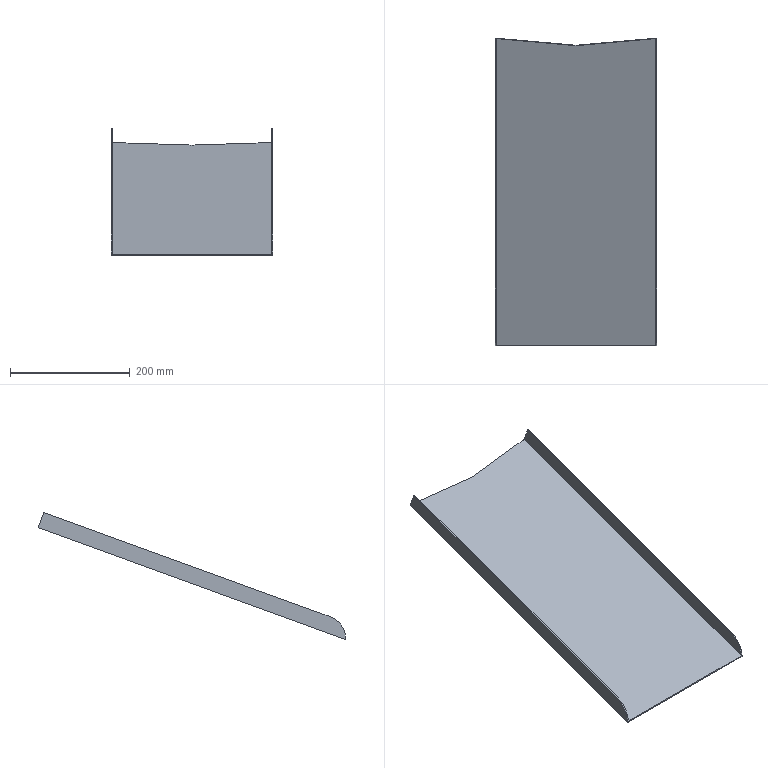Part | NX | features solid 2 | 1 solid | 17 faces | box 270 x 512.701 x 211.98 mm | volume 344500 mm3 | plane 15 | cylinder 2 | commonest cylinder face diameters 80 x2
STEP:
#1=CARTESIAN_POINT('',(133.,-620.,-424.26));
#2=VERTEX_POINT('',#1);
#3=CARTESIAN_POINT('',(-133.,-620.,-424.26));
#4=VERTEX_POINT('',#3);
#5=CARTESIAN_POINT('',(50.,-620.,-424.26));
#6=DIRECTION('',(1.,0.,0.));
#7=VECTOR('',#6,1000.);
#8=LINE('',#5,#7);
#9=EDGE_CURVE('',#2,#4,#8,.F.);
#10=ORIENTED_EDGE('',*,*,#9,.F.);
#11=CARTESIAN_POINT('',(133.,-108.158,-237.965));
#12=VERTEX_POINT('',#11);
#13=CARTESIAN_POINT('',(133.,-491.018,-377.315));
#14=DIRECTION('',(0.,-0.9397,-0.342));
#15=VECTOR('',#14,1000.);
#16=LINE('',#13,#15);
#17=EDGE_CURVE('',#12,#2,#16,.T.);
#18=ORIENTED_EDGE('',*,*,#17,.F.);
#19=CARTESIAN_POINT('',(0.,-119.794,-242.2));
#20=VERTEX_POINT('',#19);
#21=CARTESIAN_POINT('',(36.173,-116.629,-241.048));
#22=DIRECTION('',(-0.9957,-0.08711,-0.03171));
#23=VECTOR('',#22,1000.);
#24=LINE('',#21,#23);
#25=EDGE_CURVE('',#12,#20,#24,.T.);
#26=ORIENTED_EDGE('',*,*,#25,.T.);
#27=CARTESIAN_POINT('',(-133.,-108.158,-237.965));
#28=VERTEX_POINT('',#27);
#29=CARTESIAN_POINT('',(-36.173,-116.629,-241.048));
#30=DIRECTION('',(0.9957,-0.08711,-0.03171));
#31=VECTOR('',#30,1000.);
#32=LINE('',#29,#31);
#33=EDGE_CURVE('',#28,#20,#32,.T.);
#34=ORIENTED_EDGE('',*,*,#33,.F.);
#35=CARTESIAN_POINT('',(-133.,-491.018,-377.315));
#36=DIRECTION('',(0.,-0.9397,-0.342));
#37=VECTOR('',#36,1000.);
#38=LINE('',#35,#37);
#39=EDGE_CURVE('',#28,#4,#38,.T.);
#40=ORIENTED_EDGE('',*,*,#39,.T.);
#41=EDGE_LOOP('',(#10,#18,#26,#34,#40));
#42=FACE_BOUND('',#41,.T.);
#43=CARTESIAN_POINT('',(50.,-491.018,-377.315));
#44=DIRECTION('',(0.,-0.342,0.9397));
#45=DIRECTION('',(1.,0.,0.));
#46=AXIS2_PLACEMENT_3D('',#43,#44,#45);
#47=PLANE('',#46);
#48=ADVANCED_FACE('',(#42),#47,.T.);
#49=CARTESIAN_POINT('',(135.,-620.,-426.389));
#50=VERTEX_POINT('',#49);
#51=CARTESIAN_POINT('',(-135.,-620.,-426.389));
#52=VERTEX_POINT('',#51);
#53=CARTESIAN_POINT('',(50.,-620.,-426.389));
#54=DIRECTION('',(1.,0.,0.));
#55=VECTOR('',#54,1000.);
#56=LINE('',#53,#55);
#57=EDGE_CURVE('',#50,#52,#56,.F.);
#58=ORIENTED_EDGE('',*,*,#57,.F.);
#59=CARTESIAN_POINT('',(135.,-620.,-424.26));
#60=VERTEX_POINT('',#59);
#61=CARTESIAN_POINT('',(135.,-620.,-377.315));
#62=DIRECTION('',(0.,0.,1.));
#63=VECTOR('',#62,1000.);
#64=LINE('',#61,#63);
#65=EDGE_CURVE('',#60,#50,#64,.F.);
#66=ORIENTED_EDGE('',*,*,#65,.F.);
#67=CARTESIAN_POINT('',(-50.,-620.,-424.26));
#68=DIRECTION('',(1.,0.,0.));
#69=VECTOR('',#68,1000.);
#70=LINE('',#67,#69);
#71=EDGE_CURVE('',#60,#2,#70,.F.);
#72=ORIENTED_EDGE('',*,*,#71,.T.);
#73=ORIENTED_EDGE('',*,*,#9,.T.);
#74=CARTESIAN_POINT('',(-135.,-620.,-424.26));
#75=VERTEX_POINT('',#74);
#76=CARTESIAN_POINT('',(50.,-620.,-424.26));
#77=DIRECTION('',(-1.,0.,0.));
#78=VECTOR('',#77,1000.);
#79=LINE('',#76,#78);
#80=EDGE_CURVE('',#75,#4,#79,.F.);
#81=ORIENTED_EDGE('',*,*,#80,.F.);
#82=CARTESIAN_POINT('',(-135.,-620.,-377.315));
#83=DIRECTION('',(0.,0.,1.));
#84=VECTOR('',#83,1000.);
#85=LINE('',#82,#84);
#86=EDGE_CURVE('',#75,#52,#85,.F.);
#87=ORIENTED_EDGE('',*,*,#86,.T.);
#88=EDGE_LOOP('',(#58,#66,#72,#73,#81,#87));
#89=FACE_BOUND('',#88,.T.);
#90=CARTESIAN_POINT('',(50.,-620.,-570.));
#91=DIRECTION('',(0.,1.,0.));
#92=DIRECTION('',(-1.,0.,0.));
#93=AXIS2_PLACEMENT_3D('',#90,#91,#92);
#94=PLANE('',#93);
#95=ADVANCED_FACE('',(#89),#94,.F.);
#96=CARTESIAN_POINT('',(-135.,-107.299,-239.781));
#97=VERTEX_POINT('',#96);
#98=CARTESIAN_POINT('',(0.,-119.11,-244.079));
#99=VERTEX_POINT('',#98);
#100=CARTESIAN_POINT('',(-36.173,-115.945,-242.928));
#101=DIRECTION('',(0.9957,-0.08711,-0.03171));
#102=VECTOR('',#101,1000.);
#103=LINE('',#100,#102);
#104=EDGE_CURVE('',#97,#99,#103,.T.);
#105=ORIENTED_EDGE('',*,*,#104,.T.);
#106=CARTESIAN_POINT('',(135.,-107.299,-239.781));
#107=VERTEX_POINT('',#106);
#108=CARTESIAN_POINT('',(36.173,-115.945,-242.928));
#109=DIRECTION('',(-0.9957,-0.08711,-0.03171));
#110=VECTOR('',#109,1000.);
#111=LINE('',#108,#110);
#112=EDGE_CURVE('',#107,#99,#111,.T.);
#113=ORIENTED_EDGE('',*,*,#112,.F.);
#114=CARTESIAN_POINT('',(135.,-490.334,-379.194));
#115=DIRECTION('',(0.,0.9397,0.342));
#116=VECTOR('',#115,1000.);
#117=LINE('',#114,#116);
#118=EDGE_CURVE('',#107,#50,#117,.F.);
#119=ORIENTED_EDGE('',*,*,#118,.T.);
#120=ORIENTED_EDGE('',*,*,#57,.T.);
#121=CARTESIAN_POINT('',(-135.,-490.334,-379.194));
#122=DIRECTION('',(0.,0.9397,0.342));
#123=VECTOR('',#122,1000.);
#124=LINE('',#121,#123);
#125=EDGE_CURVE('',#97,#52,#124,.F.);
#126=ORIENTED_EDGE('',*,*,#125,.F.);
#127=EDGE_LOOP('',(#105,#113,#119,#120,#126));
#128=FACE_BOUND('',#127,.T.);
#129=CARTESIAN_POINT('',(50.,-490.334,-379.194));
#130=DIRECTION('',(0.,-0.342,0.9397));
#131=DIRECTION('',(1.,0.,0.));
#132=AXIS2_PLACEMENT_3D('',#129,#130,#131);
#133=PLANE('',#132);
#134=ADVANCED_FACE('',(#128),#133,.F.);
#135=ORIENTED_EDGE('',*,*,#104,.F.);
#136=CARTESIAN_POINT('',(-135.,-107.983,-237.901));
#137=VERTEX_POINT('',#136);
#138=CARTESIAN_POINT('',(-135.,-107.983,-237.901));
#139=DIRECTION('',(0.,0.342,-0.9397));
#140=VECTOR('',#139,1000.);
#141=LINE('',#138,#140);
#142=EDGE_CURVE('',#137,#97,#141,.T.);
#143=ORIENTED_EDGE('',*,*,#142,.F.);
#144=CARTESIAN_POINT('',(-36.173,-116.629,-241.048));
#145=DIRECTION('',(0.9957,-0.08711,-0.03171));
#146=VECTOR('',#145,1000.);
#147=LINE('',#144,#146);
#148=EDGE_CURVE('',#137,#28,#147,.T.);
#149=ORIENTED_EDGE('',*,*,#148,.T.);
#150=ORIENTED_EDGE('',*,*,#33,.T.);
#151=CARTESIAN_POINT('',(0.,-119.794,-242.2));
#152=DIRECTION('',(0.,0.342,-0.9397));
#153=VECTOR('',#152,1000.);
#154=LINE('',#151,#153);
#155=EDGE_CURVE('',#20,#99,#154,.T.);
#156=ORIENTED_EDGE('',*,*,#155,.T.);
#157=EDGE_LOOP('',(#135,#143,#149,#150,#156));
#158=FACE_BOUND('',#157,.T.);
#159=CARTESIAN_POINT('',(-36.173,-116.629,-241.048));
#160=DIRECTION('',(0.0927,0.9356,0.3405));
#161=DIRECTION('',(0.,-0.342,0.9397));
#162=AXIS2_PLACEMENT_3D('',#159,#160,#161);
#163=PLANE('',#162);
#164=ADVANCED_FACE('',(#158),#163,.T.);
#165=ORIENTED_EDGE('',*,*,#125,.T.);
#166=ORIENTED_EDGE('',*,*,#86,.F.);
#167=CARTESIAN_POINT('',(-135.,-593.706,-388.086));
#168=VERTEX_POINT('',#167);
#169=CARTESIAN_POINT('',(-135.,-580.025,-425.673));
#170=DIRECTION('',(-1.,0.,0.));
#171=DIRECTION('',(0.,0.,1.));
#172=AXIS2_PLACEMENT_3D('',#169,#170,#171);
#173=CIRCLE('',#172,40.);
#174=EDGE_CURVE('',#75,#168,#173,.T.);
#175=ORIENTED_EDGE('',*,*,#174,.T.);
#176=CARTESIAN_POINT('',(-135.,-116.533,-214.409));
#177=VERTEX_POINT('',#176);
#178=CARTESIAN_POINT('',(-135.,-116.533,-214.409));
#179=DIRECTION('',(0.,-0.9397,-0.342));
#180=VECTOR('',#179,1000.);
#181=LINE('',#178,#180);
#182=EDGE_CURVE('',#177,#168,#181,.T.);
#183=ORIENTED_EDGE('',*,*,#182,.F.);
#184=CARTESIAN_POINT('',(-135.,-107.983,-237.901));
#185=DIRECTION('',(0.,-0.342,0.9397));
#186=VECTOR('',#185,1000.);
#187=LINE('',#184,#186);
#188=EDGE_CURVE('',#137,#177,#187,.T.);
#189=ORIENTED_EDGE('',*,*,#188,.F.);
#190=ORIENTED_EDGE('',*,*,#142,.T.);
#191=EDGE_LOOP('',(#165,#166,#175,#183,#189,#190));
#192=FACE_BOUND('',#191,.T.);
#193=CARTESIAN_POINT('',(-135.,-491.018,-377.315));
#194=DIRECTION('',(1.,0.,0.));
#195=DIRECTION('',(0.,0.,-1.));
#196=AXIS2_PLACEMENT_3D('',#193,#194,#195);
#197=PLANE('',#196);
#198=ADVANCED_FACE('',(#192),#197,.F.);
#199=CARTESIAN_POINT('',(-133.,-107.983,-237.901));
#200=VERTEX_POINT('',#199);
#201=CARTESIAN_POINT('',(-133.,-107.983,-237.901));
#202=DIRECTION('',(0.,-0.9397,-0.342));
#203=VECTOR('',#202,1000.);
#204=LINE('',#201,#203);
#205=EDGE_CURVE('',#200,#28,#204,.T.);
#206=ORIENTED_EDGE('',*,*,#205,.T.);
#207=ORIENTED_EDGE('',*,*,#148,.F.);
#208=CARTESIAN_POINT('',(-135.,-107.983,-237.901));
#209=DIRECTION('',(1.,0.,0.));
#210=VECTOR('',#209,1000.);
#211=LINE('',#208,#210);
#212=EDGE_CURVE('',#137,#200,#211,.T.);
#213=ORIENTED_EDGE('',*,*,#212,.T.);
#214=EDGE_LOOP('',(#206,#207,#213));
#215=FACE_BOUND('',#214,.T.);
#216=CARTESIAN_POINT('',(-135.,-107.983,-237.901));
#217=DIRECTION('',(0.,0.342,-0.9397));
#218=DIRECTION('',(0.,-0.9397,-0.342));
#219=AXIS2_PLACEMENT_3D('',#216,#217,#218);
#220=PLANE('',#219);
#221=ADVANCED_FACE('',(#215),#220,.T.);
#222=ORIENTED_EDGE('',*,*,#212,.F.);
#223=ORIENTED_EDGE('',*,*,#188,.T.);
#224=CARTESIAN_POINT('',(-133.,-116.533,-214.409));
#225=VERTEX_POINT('',#224);
#226=CARTESIAN_POINT('',(-135.,-116.533,-214.409));
#227=DIRECTION('',(1.,0.,0.));
#228=VECTOR('',#227,1000.);
#229=LINE('',#226,#228);
#230=EDGE_CURVE('',#177,#225,#229,.T.);
#231=ORIENTED_EDGE('',*,*,#230,.T.);
#232=CARTESIAN_POINT('',(-133.,-107.983,-237.901));
#233=DIRECTION('',(0.,-0.342,0.9397));
#234=VECTOR('',#233,1000.);
#235=LINE('',#232,#234);
#236=EDGE_CURVE('',#200,#225,#235,.T.);
#237=ORIENTED_EDGE('',*,*,#236,.F.);
#238=EDGE_LOOP('',(#222,#223,#231,#237));
#239=FACE_BOUND('',#238,.T.);
#240=CARTESIAN_POINT('',(-135.,-107.983,-237.901));
#241=DIRECTION('',(0.,-0.9397,-0.342));
#242=DIRECTION('',(0.,-0.342,0.9397));
#243=AXIS2_PLACEMENT_3D('',#240,#241,#242);
#244=PLANE('',#243);
#245=ADVANCED_FACE('',(#239),#244,.F.);
#246=ORIENTED_EDGE('',*,*,#182,.T.);
#247=CARTESIAN_POINT('',(-133.,-593.706,-388.086));
#248=VERTEX_POINT('',#247);
#249=CARTESIAN_POINT('',(-133.,-593.706,-388.086));
#250=DIRECTION('',(-1.,0.,0.));
#251=VECTOR('',#250,1000.);
#252=LINE('',#249,#251);
#253=EDGE_CURVE('',#168,#248,#252,.F.);
#254=ORIENTED_EDGE('',*,*,#253,.T.);
#255=CARTESIAN_POINT('',(-133.,-116.533,-214.409));
#256=DIRECTION('',(0.,-0.9397,-0.342));
#257=VECTOR('',#256,1000.);
#258=LINE('',#255,#257);
#259=EDGE_CURVE('',#225,#248,#258,.T.);
#260=ORIENTED_EDGE('',*,*,#259,.F.);
#261=ORIENTED_EDGE('',*,*,#230,.F.);
#262=EDGE_LOOP('',(#246,#254,#260,#261));
#263=FACE_BOUND('',#262,.T.);
#264=CARTESIAN_POINT('',(-135.,-116.533,-214.409));
#265=DIRECTION('',(0.,0.342,-0.9397));
#266=DIRECTION('',(0.,-0.9397,-0.342));
#267=AXIS2_PLACEMENT_3D('',#264,#265,#266);
#268=PLANE('',#267);
#269=ADVANCED_FACE('',(#263),#268,.F.);
#270=ORIENTED_EDGE('',*,*,#259,.T.);
#271=CARTESIAN_POINT('',(-133.,-580.025,-425.673));
#272=DIRECTION('',(-1.,0.,0.));
#273=DIRECTION('',(0.,0.,1.));
#274=AXIS2_PLACEMENT_3D('',#271,#272,#273);
#275=CIRCLE('',#274,40.);
#276=EDGE_CURVE('',#248,#4,#275,.F.);
#277=ORIENTED_EDGE('',*,*,#276,.T.);
#278=ORIENTED_EDGE('',*,*,#39,.F.);
#279=ORIENTED_EDGE('',*,*,#205,.F.);
#280=ORIENTED_EDGE('',*,*,#236,.T.);
#281=EDGE_LOOP('',(#270,#277,#278,#279,#280));
#282=FACE_BOUND('',#281,.T.);
#283=CARTESIAN_POINT('',(-133.,-107.983,-237.901));
#284=DIRECTION('',(-1.,0.,0.));
#285=DIRECTION('',(0.,0.,1.));
#286=AXIS2_PLACEMENT_3D('',#283,#284,#285);
#287=PLANE('',#286);
#288=ADVANCED_FACE('',(#282),#287,.F.);
#289=ORIENTED_EDGE('',*,*,#174,.F.);
#290=ORIENTED_EDGE('',*,*,#80,.T.);
#291=ORIENTED_EDGE('',*,*,#276,.F.);
#292=ORIENTED_EDGE('',*,*,#253,.F.);
#293=EDGE_LOOP('',(#289,#290,#291,#292));
#294=FACE_BOUND('',#293,.T.);
#295=CARTESIAN_POINT('',(50.,-580.025,-425.673));
#296=DIRECTION('',(-1.,0.,0.));
#297=DIRECTION('',(0.,0.,1.));
#298=AXIS2_PLACEMENT_3D('',#295,#296,#297);
#299=CYLINDRICAL_SURFACE('',#298,40.);
#300=ADVANCED_FACE('',(#294),#299,.T.);
#301=ORIENTED_EDGE('',*,*,#112,.T.);
#302=ORIENTED_EDGE('',*,*,#155,.F.);
#303=ORIENTED_EDGE('',*,*,#25,.F.);
#304=CARTESIAN_POINT('',(135.,-107.983,-237.901));
#305=VERTEX_POINT('',#304);
#306=CARTESIAN_POINT('',(36.173,-116.629,-241.048));
#307=DIRECTION('',(-0.9957,-0.08711,-0.03171));
#308=VECTOR('',#307,1000.);
#309=LINE('',#306,#308);
#310=EDGE_CURVE('',#305,#12,#309,.T.);
#311=ORIENTED_EDGE('',*,*,#310,.F.);
#312=CARTESIAN_POINT('',(135.,-107.983,-237.901));
#313=DIRECTION('',(0.,0.342,-0.9397));
#314=VECTOR('',#313,1000.);
#315=LINE('',#312,#314);
#316=EDGE_CURVE('',#305,#107,#315,.T.);
#317=ORIENTED_EDGE('',*,*,#316,.T.);
#318=EDGE_LOOP('',(#301,#302,#303,#311,#317));
#319=FACE_BOUND('',#318,.T.);
#320=CARTESIAN_POINT('',(36.173,-116.629,-241.048));
#321=DIRECTION('',(-0.0927,0.9356,0.3405));
#322=DIRECTION('',(0.,-0.342,0.9397));
#323=AXIS2_PLACEMENT_3D('',#320,#321,#322);
#324=PLANE('',#323);
#325=ADVANCED_FACE('',(#319),#324,.T.);
#326=ORIENTED_EDGE('',*,*,#118,.F.);
#327=ORIENTED_EDGE('',*,*,#316,.F.);
#328=CARTESIAN_POINT('',(135.,-116.533,-214.409));
#329=VERTEX_POINT('',#328);
#330=CARTESIAN_POINT('',(135.,-107.983,-237.901));
#331=DIRECTION('',(0.,-0.342,0.9397));
#332=VECTOR('',#331,1000.);
#333=LINE('',#330,#332);
#334=EDGE_CURVE('',#305,#329,#333,.T.);
#335=ORIENTED_EDGE('',*,*,#334,.T.);
#336=CARTESIAN_POINT('',(135.,-593.706,-388.086));
#337=VERTEX_POINT('',#336);
#338=CARTESIAN_POINT('',(135.,-116.533,-214.409));
#339=DIRECTION('',(0.,-0.9397,-0.342));
#340=VECTOR('',#339,1000.);
#341=LINE('',#338,#340);
#342=EDGE_CURVE('',#329,#337,#341,.T.);
#343=ORIENTED_EDGE('',*,*,#342,.T.);
#344=CARTESIAN_POINT('',(135.,-580.025,-425.673));
#345=DIRECTION('',(-1.,0.,0.));
#346=DIRECTION('',(0.,0.,1.));
#347=AXIS2_PLACEMENT_3D('',#344,#345,#346);
#348=CIRCLE('',#347,40.);
#349=EDGE_CURVE('',#60,#337,#348,.T.);
#350=ORIENTED_EDGE('',*,*,#349,.F.);
#351=ORIENTED_EDGE('',*,*,#65,.T.);
#352=EDGE_LOOP('',(#326,#327,#335,#343,#350,#351));
#353=FACE_BOUND('',#352,.T.);
#354=CARTESIAN_POINT('',(135.,-491.018,-377.315));
#355=DIRECTION('',(-1.,0.,0.));
#356=DIRECTION('',(0.,0.,-1.));
#357=AXIS2_PLACEMENT_3D('',#354,#355,#356);
#358=PLANE('',#357);
#359=ADVANCED_FACE('',(#353),#358,.F.);
#360=CARTESIAN_POINT('',(133.,-107.983,-237.901));
#361=VERTEX_POINT('',#360);
#362=CARTESIAN_POINT('',(133.,-107.983,-237.901));
#363=DIRECTION('',(0.,-0.9397,-0.342));
#364=VECTOR('',#363,1000.);
#365=LINE('',#362,#364);
#366=EDGE_CURVE('',#361,#12,#365,.T.);
#367=ORIENTED_EDGE('',*,*,#366,.F.);
#368=CARTESIAN_POINT('',(135.,-107.983,-237.901));
#369=DIRECTION('',(-1.,0.,0.));
#370=VECTOR('',#369,1000.);
#371=LINE('',#368,#370);
#372=EDGE_CURVE('',#305,#361,#371,.T.);
#373=ORIENTED_EDGE('',*,*,#372,.F.);
#374=ORIENTED_EDGE('',*,*,#310,.T.);
#375=EDGE_LOOP('',(#367,#373,#374));
#376=FACE_BOUND('',#375,.T.);
#377=CARTESIAN_POINT('',(135.,-107.983,-237.901));
#378=DIRECTION('',(0.,0.342,-0.9397));
#379=DIRECTION('',(0.,-0.9397,-0.342));
#380=AXIS2_PLACEMENT_3D('',#377,#378,#379);
#381=PLANE('',#380);
#382=ADVANCED_FACE('',(#376),#381,.T.);
#383=ORIENTED_EDGE('',*,*,#372,.T.);
#384=CARTESIAN_POINT('',(133.,-116.533,-214.409));
#385=VERTEX_POINT('',#384);
#386=CARTESIAN_POINT('',(133.,-107.983,-237.901));
#387=DIRECTION('',(0.,-0.342,0.9397));
#388=VECTOR('',#387,1000.);
#389=LINE('',#386,#388);
#390=EDGE_CURVE('',#361,#385,#389,.T.);
#391=ORIENTED_EDGE('',*,*,#390,.T.);
#392=CARTESIAN_POINT('',(135.,-116.533,-214.409));
#393=DIRECTION('',(-1.,0.,0.));
#394=VECTOR('',#393,1000.);
#395=LINE('',#392,#394);
#396=EDGE_CURVE('',#329,#385,#395,.T.);
#397=ORIENTED_EDGE('',*,*,#396,.F.);
#398=ORIENTED_EDGE('',*,*,#334,.F.);
#399=EDGE_LOOP('',(#383,#391,#397,#398));
#400=FACE_BOUND('',#399,.T.);
#401=CARTESIAN_POINT('',(135.,-107.983,-237.901));
#402=DIRECTION('',(0.,-0.9397,-0.342));
#403=DIRECTION('',(0.,-0.342,0.9397));
#404=AXIS2_PLACEMENT_3D('',#401,#402,#403);
#405=PLANE('',#404);
#406=ADVANCED_FACE('',(#400),#405,.F.);
#407=ORIENTED_EDGE('',*,*,#342,.F.);
#408=ORIENTED_EDGE('',*,*,#396,.T.);
#409=CARTESIAN_POINT('',(133.,-593.706,-388.086));
#410=VERTEX_POINT('',#409);
#411=CARTESIAN_POINT('',(133.,-116.533,-214.409));
#412=DIRECTION('',(0.,-0.9397,-0.342));
#413=VECTOR('',#412,1000.);
#414=LINE('',#411,#413);
#415=EDGE_CURVE('',#385,#410,#414,.T.);
#416=ORIENTED_EDGE('',*,*,#415,.T.);
#417=CARTESIAN_POINT('',(133.,-593.706,-388.086));
#418=DIRECTION('',(1.,0.,0.));
#419=VECTOR('',#418,1000.);
#420=LINE('',#417,#419);
#421=EDGE_CURVE('',#337,#410,#420,.F.);
#422=ORIENTED_EDGE('',*,*,#421,.F.);
#423=EDGE_LOOP('',(#407,#408,#416,#422));
#424=FACE_BOUND('',#423,.T.);
#425=CARTESIAN_POINT('',(135.,-116.533,-214.409));
#426=DIRECTION('',(0.,0.342,-0.9397));
#427=DIRECTION('',(0.,-0.9397,-0.342));
#428=AXIS2_PLACEMENT_3D('',#425,#426,#427);
#429=PLANE('',#428);
#430=ADVANCED_FACE('',(#424),#429,.F.);
#431=ORIENTED_EDGE('',*,*,#415,.F.);
#432=ORIENTED_EDGE('',*,*,#390,.F.);
#433=ORIENTED_EDGE('',*,*,#366,.T.);
#434=ORIENTED_EDGE('',*,*,#17,.T.);
#435=CARTESIAN_POINT('',(133.,-580.025,-425.673));
#436=DIRECTION('',(-1.,0.,0.));
#437=DIRECTION('',(0.,0.,1.));
#438=AXIS2_PLACEMENT_3D('',#435,#436,#437);
#439=CIRCLE('',#438,40.);
#440=EDGE_CURVE('',#410,#2,#439,.F.);
#441=ORIENTED_EDGE('',*,*,#440,.F.);
#442=EDGE_LOOP('',(#431,#432,#433,#434,#441));
#443=FACE_BOUND('',#442,.T.);
#444=CARTESIAN_POINT('',(133.,-107.983,-237.901));
#445=DIRECTION('',(1.,0.,0.));
#446=DIRECTION('',(0.,0.,1.));
#447=AXIS2_PLACEMENT_3D('',#444,#445,#446);
#448=PLANE('',#447);
#449=ADVANCED_FACE('',(#443),#448,.F.);
#450=ORIENTED_EDGE('',*,*,#349,.T.);
#451=ORIENTED_EDGE('',*,*,#421,.T.);
#452=ORIENTED_EDGE('',*,*,#440,.T.);
#453=ORIENTED_EDGE('',*,*,#71,.F.);
#454=EDGE_LOOP('',(#450,#451,#452,#453));
#455=FACE_BOUND('',#454,.T.);
#456=CARTESIAN_POINT('',(-50.,-580.025,-425.673));
#457=DIRECTION('',(1.,0.,0.));
#458=DIRECTION('',(0.,0.,1.));
#459=AXIS2_PLACEMENT_3D('',#456,#457,#458);
#460=CYLINDRICAL_SURFACE('',#459,40.);
#461=ADVANCED_FACE('',(#455),#460,.T.);
#462=CLOSED_SHELL('',(#48,#95,#134,#164,#198,#221,#245,#269,#288,#300,#325,#359,#382,#406,#430,#449,#461));
#463=MANIFOLD_SOLID_BREP('',#462);
#464=(LENGTH_UNIT()NAMED_UNIT(*)SI_UNIT(.MILLI.,.METRE.));
#465=UNCERTAINTY_MEASURE_WITH_UNIT(LENGTH_MEASURE(0.00001),#464,'','');
#466=(NAMED_UNIT(*)PLANE_ANGLE_UNIT()SI_UNIT($,.RADIAN.));
#467=(NAMED_UNIT(*)SI_UNIT($,.STERADIAN.)SOLID_ANGLE_UNIT());
#468=(GEOMETRIC_REPRESENTATION_CONTEXT(3)GLOBAL_UNCERTAINTY_ASSIGNED_CONTEXT((#465))GLOBAL_UNIT_ASSIGNED_CONTEXT((#464,#466,#467))REPRESENTATION_CONTEXT('',''));
#469=ADVANCED_BREP_SHAPE_REPRESENTATION('',(#463),#468);